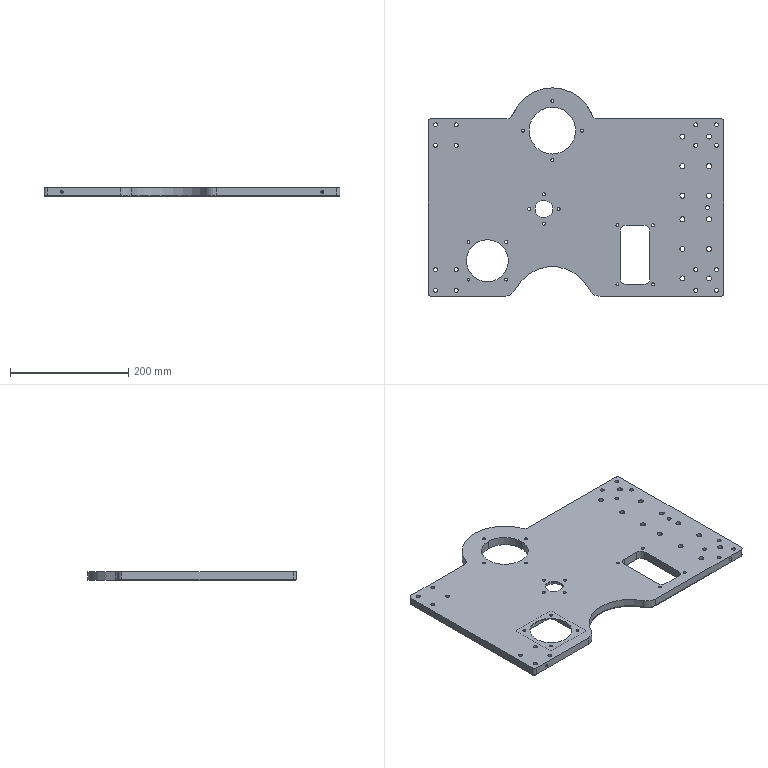NC program | Mastercam | posted with a generic post
Lines 1 to 790 of 11903:
%
O0000()
(MATERIAL - ALUMINUM MM - 2024)
( T20 | 20 FEM | H20 | XY STOCK TO LEAVE - .1 | Z STOCK TO LEAVE - .03 )
( T16 | 16 FEM | H16 | XY STOCK TO LEAVE - 0. | Z STOCK TO LEAVE - .03 )
( T8 | 8 FEM | H8 | XY STOCK TO LEAVE - .1 | Z STOCK TO LEAVE - .2 )
( T4 | 4 FEM | H4 | XY STOCK TO LEAVE - .05 | Z STOCK TO LEAVE - .2 )
( T7 | 4 CHM | H7 )
( T18 | 8.5 DR | H18 )
( T14 | 6.8 DR | H14 )
( T1 | 5 DR | H1 )
( T9 | 6.6 DR | H9 )
( T6 | 6 FEM | H6 | XY STOCK TO LEAVE - .07 | Z STOCK TO LEAVE - .05 )
( T11 | 8 BNOS | H11 )
( T3 | 10.5 DR | H3 )
N100 G21
N110 G0 G17 G40 G49 G80 G90
( YDICL )
N120 T20 M6
N130 G0 G90 G54 X260.1 Y191.25 A0. S5000 M3
N140 G43 H20 Z50. M8
N150 Z1.1
N160 G1 Z-1.784 F600.
N170 Y171.25 F4000.
N180 Y-171.75
N190 Y-191.75
N200 Z-3.667 F600.
N210 Y-171.75 F4000.
N220 Y171.25
N230 Y191.25
N240 Z-5.551 F600.
N250 Y171.25 F4000.
N260 Y-171.75
N270 Y-191.75
N280 Z-7.435 F600.
N290 Y-171.75 F4000.
N300 Y171.25
N310 Y191.25
N320 Z-9.319 F600.
N330 Y171.25 F4000.
N340 Y-171.75
N350 Y-191.75
N360 Z-11.203 F600.
N370 Y-171.75 F4000.
N380 Y171.25
N390 Y191.25
N400 Z-13.086 F600.
N410 Y171.25 F4000.
N420 Y-171.75
N430 Y-191.75
N440 Z-14.97 F600.
N450 Y-171.75 F4000.
N460 Y171.25
N470 Y191.25
N480 G0 Z50.
N490 X-260.1 Y-191.75
N500 Z1.1
N510 G1 Z-1.784 F600.
N520 Y-171.75 F4000.
N530 Y171.25
N540 Y191.25
N550 Z-3.667 F600.
N560 Y171.25 F4000.
N570 Y-171.75
N580 Y-191.75
N590 Z-5.551 F600.
N600 Y-171.75 F4000.
N610 Y171.25
N620 Y191.25
N630 Z-7.435 F600.
N640 Y171.25 F4000.
N650 Y-171.75
N660 Y-191.75
N670 Z-9.319 F600.
N680 Y-171.75 F4000.
N690 Y171.25
N700 Y191.25
N710 Z-11.203 F600.
N720 Y171.25 F4000.
N730 Y-171.75
N740 Y-191.75
N750 Z-13.086 F600.
N760 Y-171.75 F4000.
N770 Y171.25
N780 Y191.25
N790 Z-14.97 F600.
N800 Y171.25 F4000.
N810 Y-171.75
N820 Y-191.75
N830 G0 Z50.
N840 X-40. Y-93.85
N850 Z1.1
N860 G1 Z.1 F600.
N870 G3 X-49.9 Y-103.75 Z-.15 I0. J-9.9 F4000.
N880 X-40. Y-113.65 Z-.4 I9.9 J0.
N890 X-30.1 Y-103.75 Z-.65 I0. J9.9
N900 X-40. Y-93.85 Z-.9 I-9.9 J0.
N910 X-49.9 Y-103.75 Z-1.15 I0. J-9.9
N920 X-40. Y-113.65 Z-1.4 I9.9 J0.
N930 X-30.1 Y-103.75 Z-1.65 I0. J9.9
N940 X-40. Y-93.85 Z-1.9 I-9.9 J0.
N950 X-49.9 Y-103.75 Z-2.15 I0. J-9.9
N960 X-40. Y-113.65 Z-2.4 I9.9 J0.
N970 X-30.1 Y-103.75 Z-2.65 I0. J9.9
N980 X-40. Y-93.85 Z-2.9 I-9.9 J0.
N990 X-49.9 Y-103.75 Z-3.15 I0. J-9.9
N1000 X-40. Y-113.65 Z-3.4 I9.9 J0.
N1010 X-30.1 Y-103.75 Z-3.65 I0. J9.9
N1020 X-40. Y-93.85 Z-3.9 I-9.9 J0.
N1030 X-49.9 Y-103.75 Z-4.15 I0. J-9.9
N1040 X-40. Y-113.65 Z-4.4 I9.9 J0.
N1050 X-30.1 Y-103.75 Z-4.65 I0. J9.9
N1060 X-40. Y-93.85 Z-4.9 I-9.9 J0.
N1070 X-49.9 Y-103.75 Z-5.15 I0. J-9.9
N1080 X-40. Y-113.65 Z-5.4 I9.9 J0.
N1090 X-30.1 Y-103.75 Z-5.65 I0. J9.9
N1100 X-40. Y-93.85 Z-5.9 I-9.9 J0.
N1110 X-49.9 Y-103.75 Z-6.15 I0. J-9.9
N1120 X-40. Y-113.65 Z-6.4 I9.9 J0.
N1130 X-30.1 Y-103.75 Z-6.65 I0. J9.9
N1140 X-40. Y-93.85 Z-6.9 I-9.9 J0.
N1150 X-49.9 Y-103.75 Z-7.15 I0. J-9.9
N1160 X-40. Y-113.65 Z-7.4 I9.9 J0.
N1170 X-30.1 Y-103.75 Z-7.65 I0. J9.9
N1180 X-40. Y-93.85 Z-7.9 I-9.9 J0.
N1190 X-49.9 Y-103.75 Z-8.15 I0. J-9.9
N1200 X-40. Y-113.65 Z-8.4 I9.9 J0.
N1210 X-30.1 Y-103.75 Z-8.65 I0. J9.9
N1220 X-40. Y-93.85 Z-8.9 I-9.9 J0.
N1230 X-49.9 Y-103.75 Z-9.15 I0. J-9.9
N1240 X-40. Y-113.65 Z-9.4 I9.9 J0.
N1250 X-30.1 Y-103.75 Z-9.65 I0. J9.9
N1260 X-40. Y-93.85 Z-9.9 I-9.9 J0.
N1270 X-49.9 Y-103.75 Z-10.15 I0. J-9.9
N1280 X-40. Y-113.65 Z-10.4 I9.9 J0.
N1290 X-30.1 Y-103.75 Z-10.65 I0. J9.9
N1300 X-40. Y-93.85 Z-10.9 I-9.9 J0.
N1310 X-49.9 Y-103.75 Z-11.15 I0. J-9.9
N1320 X-40. Y-113.65 Z-11.4 I9.9 J0.
N1330 X-30.1 Y-103.75 Z-11.65 I0. J9.9
N1340 X-40. Y-93.85 Z-11.9 I-9.9 J0.
N1350 X-49.9 Y-103.75 Z-12.15 I0. J-9.9
N1360 X-40. Y-113.65 Z-12.4 I9.9 J0.
N1370 X-30.1 Y-103.75 Z-12.65 I0. J9.9
N1380 X-40. Y-93.85 Z-12.9 I-9.9 J0.
N1390 X-49.9 Y-103.75 Z-13.15 I0. J-9.9
N1400 X-40. Y-113.65 Z-13.4 I9.9 J0.
N1410 X-30.1 Y-103.75 Z-13.65 I0. J9.9
N1420 X-40. Y-93.85 Z-13.9 I-9.9 J0.
N1430 X-49.9 Y-103.75 Z-14.15 I0. J-9.9
N1440 X-40. Y-113.65 Z-14.4 I9.9 J0.
N1450 X-30.1 Y-103.75 Z-14.65 I0. J9.9
N1460 X-40. Y-93.85 Z-14.9 I-9.9 J0.
N1470 X-44.215 Y-94.792 Z-14.97 I0. J-9.9
N1480 X-49.9 Y-103.75 I4.215 J-8.958
N1490 X-40. Y-113.65 I9.9 J0.
N1500 X-30.1 Y-103.75 I0. J9.9
N1510 X-40. Y-93.85 I-9.9 J0.
N1520 X-44.662 Y-95.016 I0. J-9.9
N1530 G0 Z50.
N1540 X-40. Y-74.35
N1550 Z1.1
N1560 G1 Z.1 F600.
N1570 G3 X-69.4 Y-103.75 Z-.15 I0. J-29.4 F4000.
N1580 X-40. Y-133.15 Z-.4 I29.4 J0.
N1590 X-10.6 Y-103.75 Z-.65 I0. J29.4
N1600 X-40. Y-74.35 Z-.9 I-29.4 J0.
N1610 X-69.4 Y-103.75 Z-1.15 I0. J-29.4
N1620 X-40. Y-133.15 Z-1.4 I29.4 J0.
N1630 X-10.6 Y-103.75 Z-1.65 I0. J29.4
N1640 X-40. Y-74.35 Z-1.9 I-29.4 J0.
N1650 X-69.4 Y-103.75 Z-2.15 I0. J-29.4
N1660 X-40. Y-133.15 Z-2.4 I29.4 J0.
N1670 X-10.6 Y-103.75 Z-2.65 I0. J29.4
N1680 X-40. Y-74.35 Z-2.9 I-29.4 J0.
N1690 X-69.4 Y-103.75 Z-3.15 I0. J-29.4
N1700 X-40. Y-133.15 Z-3.4 I29.4 J0.
N1710 X-10.6 Y-103.75 Z-3.65 I0. J29.4
N1720 X-40. Y-74.35 Z-3.9 I-29.4 J0.
N1730 X-69.4 Y-103.75 Z-4.15 I0. J-29.4
N1740 X-40. Y-133.15 Z-4.4 I29.4 J0.
N1750 X-10.6 Y-103.75 Z-4.65 I0. J29.4
N1760 X-40. Y-74.35 Z-4.9 I-29.4 J0.
N1770 X-69.4 Y-103.75 Z-5.15 I0. J-29.4
N1780 X-40. Y-133.15 Z-5.4 I29.4 J0.
N1790 X-10.6 Y-103.75 Z-5.65 I0. J29.4
N1800 X-40. Y-74.35 Z-5.9 I-29.4 J0.
N1810 X-69.4 Y-103.75 Z-6.15 I0. J-29.4
N1820 X-40. Y-133.15 Z-6.4 I29.4 J0.
N1830 X-10.6 Y-103.75 Z-6.65 I0. J29.4
N1840 X-40. Y-74.35 Z-6.9 I-29.4 J0.
N1850 X-69.4 Y-103.75 Z-7.15 I0. J-29.4
N1860 X-40. Y-133.15 Z-7.4 I29.4 J0.
N1870 X-10.6 Y-103.75 Z-7.65 I0. J29.4
N1880 X-40. Y-74.35 Z-7.9 I-29.4 J0.
N1890 X-69.4 Y-103.75 Z-8.15 I0. J-29.4
N1900 X-40. Y-133.15 Z-8.4 I29.4 J0.
N1910 X-10.6 Y-103.75 Z-8.65 I0. J29.4
N1920 X-40. Y-74.35 Z-8.9 I-29.4 J0.
N1930 X-69.4 Y-103.75 Z-9.15 I0. J-29.4
N1940 X-40. Y-133.15 Z-9.4 I29.4 J0.
N1950 X-10.6 Y-103.75 Z-9.65 I0. J29.4
N1960 X-40. Y-74.35 Z-9.9 I-29.4 J0.
N1970 X-69.4 Y-103.75 Z-10.15 I0. J-29.4
N1980 X-40. Y-133.15 Z-10.4 I29.4 J0.
N1990 X-10.6 Y-103.75 Z-10.65 I0. J29.4
N2000 X-40. Y-74.35 Z-10.9 I-29.4 J0.
N2010 X-69.4 Y-103.75 Z-11.15 I0. J-29.4
N2020 X-40. Y-133.15 Z-11.4 I29.4 J0.
N2030 X-10.6 Y-103.75 Z-11.65 I0. J29.4
N2040 X-40. Y-74.35 Z-11.9 I-29.4 J0.
N2050 X-69.4 Y-103.75 Z-12.15 I0. J-29.4
N2060 X-40. Y-133.15 Z-12.4 I29.4 J0.
N2070 X-10.6 Y-103.75 Z-12.65 I0. J29.4
N2080 X-40. Y-74.35 Z-12.9 I-29.4 J0.
N2090 X-69.4 Y-103.75 Z-13.15 I0. J-29.4
N2100 X-40. Y-133.15 Z-13.4 I29.4 J0.
N2110 X-10.6 Y-103.75 Z-13.65 I0. J29.4
N2120 X-40. Y-74.35 Z-13.9 I-29.4 J0.
N2130 X-69.4 Y-103.75 Z-14.15 I0. J-29.4
N2140 X-40. Y-133.15 Z-14.4 I29.4 J0.
N2150 X-10.6 Y-103.75 Z-14.65 I0. J29.4
N2160 X-40. Y-74.35 Z-14.9 I-29.4 J0.
N2170 X-52.518 Y-77.148 Z-14.97 I0. J-29.4
N2180 X-69.4 Y-103.75 I12.518 J-26.602
N2190 X-40. Y-133.15 I29.4 J0.
N2200 X-10.6 Y-103.75 I0. J29.4
N2210 X-40. Y-74.35 I-29.4 J0.
N2220 X-52.968 Y-77.365 I0. J-29.4
N2230 G0 Z50.
N2240 X106.9 Y138.15
N2250 Z1.1
N2260 G1 Z.1 F600.
N2270 X93.1 Z.011 F4000.
N2280 Y74.35 Z-.4
N2290 X106.9 Z-.489
N2300 Y138.15 Z-.9
N2310 X93.1 Z-.989
N2320 Y74.35 Z-1.4
N2330 X106.9 Z-1.489
N2340 Y138.15 Z-1.9
N2350 X93.1 Z-1.989
N2360 Y74.35 Z-2.4
N2370 X106.9 Z-2.489
N2380 Y138.15 Z-2.9
N2390 X93.1 Z-2.989
N2400 Y74.35 Z-3.4
N2410 X106.9 Z-3.489
N2420 Y138.15 Z-3.9
N2430 X93.1 Z-3.989
N2440 Y74.35 Z-4.4
N2450 X106.9 Z-4.489
N2460 Y138.15 Z-4.9
N2470 X93.1 Z-4.989
N2480 Y74.35 Z-5.4
N2490 X106.9 Z-5.489
N2500 Y138.15 Z-5.9
N2510 X93.1 Z-5.989
N2520 Y74.35 Z-6.4
N2530 X106.9 Z-6.489
N2540 Y138.15 Z-6.9
N2550 X93.1 Z-6.989
N2560 Y74.35 Z-7.4
N2570 X106.9 Z-7.489
N2580 Y138.15 Z-7.9
N2590 X93.1 Z-7.989
N2600 Y74.35 Z-8.4
N2610 X106.9 Z-8.489
N2620 Y138.15 Z-8.9
N2630 X93.1 Z-8.989
N2640 Y74.35 Z-9.4
N2650 X106.9 Z-9.489
N2660 Y138.15 Z-9.9
N2670 X93.1 Z-9.989
N2680 Y74.35 Z-10.4
N2690 X106.9 Z-10.489
N2700 Y138.15 Z-10.9
N2710 X93.1 Z-10.989
N2720 Y74.35 Z-11.4
N2730 X106.9 Z-11.489
N2740 Y138.15 Z-11.9
N2750 X93.1 Z-11.989
N2760 Y74.35 Z-12.4
N2770 X106.9 Z-12.489
N2780 Y138.15 Z-12.9
N2790 X93.1 Z-12.989
N2800 Y74.35 Z-13.4
N2810 X106.9 Z-13.489
N2820 Y138.15 Z-13.9
N2830 X93.1 Z-13.989
N2840 Y74.35 Z-14.4
N2850 X106.9 Z-14.489
N2860 Y138.15 Z-14.9
N2870 X96.036 Z-14.97
N2880 X93.1
N2890 Y74.35
N2900 X106.9
N2910 Y138.15
N2920 X95.536
N2930 G0 Z50.
N2940 X114.9 Y146.15
N2950 Z1.1
N2960 G1 Z.1 F600.
N2970 X85.1 Z-.036 F4000.
N2980 Y66.35 Z-.4
N2990 X114.9 Z-.536
N3000 Y146.15 Z-.9
N3010 X85.1 Z-1.036
N3020 Y66.35 Z-1.4
N3030 X114.9 Z-1.536
N3040 Y146.15 Z-1.9
N3050 X85.1 Z-2.036
N3060 Y66.35 Z-2.4
N3070 X114.9 Z-2.536
N3080 Y146.15 Z-2.9
N3090 X85.1 Z-3.036
N3100 Y66.35 Z-3.4
N3110 X114.9 Z-3.536
N3120 Y146.15 Z-3.9
N3130 X85.1 Z-4.036
N3140 Y66.35 Z-4.4
N3150 X114.9 Z-4.536
N3160 Y146.15 Z-4.9
N3170 X85.1 Z-5.036
N3180 Y66.35 Z-5.4
N3190 X114.9 Z-5.536
N3200 Y146.15 Z-5.9
N3210 X85.1 Z-6.036
N3220 Y66.35 Z-6.4
N3230 X114.9 Z-6.536
N3240 Y146.15 Z-6.9
N3250 X85.1 Z-7.036
N3260 Y66.35 Z-7.4
N3270 X114.9 Z-7.536
N3280 Y146.15 Z-7.9
N3290 X85.1 Z-8.036
N3300 Y66.35 Z-8.4
N3310 X114.9 Z-8.536
N3320 Y146.15 Z-8.9
N3330 X85.1 Z-9.036
N3340 Y66.35 Z-9.4
N3350 X114.9 Z-9.536
N3360 Y146.15 Z-9.9
N3370 X85.1 Z-10.036
N3380 Y66.35 Z-10.4
N3390 X114.9 Z-10.536
N3400 Y146.15 Z-10.9
N3410 X85.1 Z-11.036
N3420 Y66.35 Z-11.4
N3430 X114.9 Z-11.536
N3440 Y146.15 Z-11.9
N3450 X85.1 Z-12.036
N3460 Y66.35 Z-12.4
N3470 X114.9 Z-12.536
N3480 Y146.15 Z-12.9
N3490 X85.1 Z-13.036
N3500 Y66.35 Z-13.4
N3510 X114.9 Z-13.536
N3520 Y146.15 Z-13.9
N3530 X85.1 Z-14.036
N3540 Y66.35 Z-14.4
N3550 X114.9 Z-14.536
N3560 Y146.15 Z-14.9
N3570 X99.556 Z-14.97
N3580 X85.1
N3590 Y66.35
N3600 X114.9
N3610 Y146.15
N3620 X99.056
N3630 G0 Z50.
N3640 X-54.364 Y33.668
N3650 Z1.1
N3660 G1 Z.1 F600.
N3670 G3 X-59.264 Y28.768 Z-.15 I0. J-4.9 F3000.
N3680 X-54.364 Y23.868 Z-.4 I4.9 J0.
N3690 X-49.464 Y28.768 Z-.65 I0. J4.9
N3700 X-54.364 Y33.668 Z-.9 I-4.9 J0.
N3710 X-59.264 Y28.768 Z-1.15 I0. J-4.9
N3720 X-54.364 Y23.868 Z-1.4 I4.9 J0.
N3730 X-49.464 Y28.768 Z-1.65 I0. J4.9
N3740 X-54.364 Y33.668 Z-1.9 I-4.9 J0.
N3750 X-59.264 Y28.768 Z-2.15 I0. J-4.9
N3760 X-54.364 Y23.868 Z-2.4 I4.9 J0.
N3770 X-49.464 Y28.768 Z-2.65 I0. J4.9
N3780 X-54.364 Y33.668 Z-2.9 I-4.9 J0.
N3790 X-59.264 Y28.768 Z-3.15 I0. J-4.9
N3800 X-54.364 Y23.868 Z-3.4 I4.9 J0.
N3810 X-49.464 Y28.768 Z-3.65 I0. J4.9
N3820 X-54.364 Y33.668 Z-3.9 I-4.9 J0.
N3830 X-59.264 Y28.768 Z-4.15 I0. J-4.9
N3840 X-54.364 Y23.868 Z-4.4 I4.9 J0.
N3850 X-49.464 Y28.768 Z-4.65 I0. J4.9
N3860 X-54.364 Y33.668 Z-4.9 I-4.9 J0.
N3870 X-59.264 Y28.768 Z-5.15 I0. J-4.9
N3880 X-54.364 Y23.868 Z-5.4 I4.9 J0.
N3890 X-49.464 Y28.768 Z-5.65 I0. J4.9
N3900 X-54.364 Y33.668 Z-5.9 I-4.9 J0.
N3910 X-59.264 Y28.768 Z-6.15 I0. J-4.9
N3920 X-54.364 Y23.868 Z-6.4 I4.9 J0.
N3930 X-49.464 Y28.768 Z-6.65 I0. J4.9
N3940 X-54.364 Y33.668 Z-6.9 I-4.9 J0.
N3950 X-59.264 Y28.768 Z-7.15 I0. J-4.9
N3960 X-54.364 Y23.868 Z-7.4 I4.9 J0.
N3970 X-49.464 Y28.768 Z-7.65 I0. J4.9
N3980 X-54.364 Y33.668 Z-7.9 I-4.9 J0.
N3990 X-59.264 Y28.768 Z-8.15 I0. J-4.9
N4000 X-54.364 Y23.868 Z-8.4 I4.9 J0.
N4010 X-49.464 Y28.768 Z-8.65 I0. J4.9
N4020 X-54.364 Y33.668 Z-8.9 I-4.9 J0.
N4030 X-59.264 Y28.768 Z-9.15 I0. J-4.9
N4040 X-54.364 Y23.868 Z-9.4 I4.9 J0.
N4050 X-49.464 Y28.768 Z-9.65 I0. J4.9
N4060 X-54.364 Y33.668 Z-9.9 I-4.9 J0.
N4070 X-59.264 Y28.768 Z-10.15 I0. J-4.9
N4080 X-54.364 Y23.868 Z-10.4 I4.9 J0.
N4090 X-49.464 Y28.768 Z-10.65 I0. J4.9
N4100 X-54.364 Y33.668 Z-10.9 I-4.9 J0.
N4110 X-59.264 Y28.768 Z-11.15 I0. J-4.9
N4120 X-54.364 Y23.868 Z-11.4 I4.9 J0.
N4130 X-49.464 Y28.768 Z-11.65 I0. J4.9
N4140 X-54.364 Y33.668 Z-11.9 I-4.9 J0.
N4150 X-59.264 Y28.768 Z-12.15 I0. J-4.9
N4160 X-54.364 Y23.868 Z-12.4 I4.9 J0.
N4170 X-49.464 Y28.768 Z-12.65 I0. J4.9
N4180 X-54.364 Y33.668 Z-12.9 I-4.9 J0.
N4190 X-59.264 Y28.768 Z-13.15 I0. J-4.9
N4200 X-54.364 Y23.868 Z-13.4 I4.9 J0.
N4210 X-49.464 Y28.768 Z-13.65 I0. J4.9
N4220 X-54.364 Y33.668 Z-13.9 I-4.9 J0.
N4230 X-59.264 Y28.768 Z-14.15 I0. J-4.9
N4240 X-54.364 Y23.868 Z-14.4 I4.9 J0.
N4250 X-49.464 Y28.768 Z-14.65 I0. J4.9
N4260 X-54.364 Y33.668 Z-14.9 I-4.9 J0.
N4270 X-56.45 Y33.201 Z-14.97 I0. J-4.9
N4280 X-59.263 Y28.768 I2.086 J-4.433
N4290 X-54.364 Y23.869 I4.899 J0.
N4300 X-49.465 Y28.768 I0. J4.899
N4310 X-54.364 Y33.668 I-4.899 J0.
N4320 X-56.891 Y32.966 I0. J-4.9
N4330 G0 Z50.
N4340 X-54.364 Y37.168
N4350 Z1.1
N4360 G1 Z.1 F600.
N4370 G3 X-62.764 Y28.768 Z-.15 I0. J-8.4 F3000.
N4380 X-54.364 Y20.368 Z-.4 I8.4 J0.
N4390 X-45.964 Y28.768 Z-.65 I0. J8.4
N4400 X-54.364 Y37.168 Z-.9 I-8.4 J0.
N4410 X-62.764 Y28.768 Z-1.15 I0. J-8.4
N4420 X-54.364 Y20.368 Z-1.4 I8.4 J0.
N4430 X-45.964 Y28.768 Z-1.65 I0. J8.4
N4440 X-54.364 Y37.168 Z-1.9 I-8.4 J0.
N4450 X-62.764 Y28.768 Z-2.15 I0. J-8.4
N4460 X-54.364 Y20.368 Z-2.4 I8.4 J0.
N4470 X-45.964 Y28.768 Z-2.65 I0. J8.4
N4480 X-54.364 Y37.168 Z-2.9 I-8.4 J0.
N4490 X-62.764 Y28.768 Z-3.15 I0. J-8.4
N4500 X-54.364 Y20.368 Z-3.4 I8.4 J0.
N4510 X-45.964 Y28.768 Z-3.65 I0. J8.4
N4520 X-54.364 Y37.168 Z-3.9 I-8.4 J0.
N4530 X-62.764 Y28.768 Z-4.15 I0. J-8.4
N4540 X-54.364 Y20.368 Z-4.4 I8.4 J0.
N4550 X-45.964 Y28.768 Z-4.65 I0. J8.4
N4560 X-54.364 Y37.168 Z-4.9 I-8.4 J0.
N4570 X-62.764 Y28.768 Z-5.15 I0. J-8.4
N4580 X-54.364 Y20.368 Z-5.4 I8.4 J0.
N4590 X-45.964 Y28.768 Z-5.65 I0. J8.4
N4600 X-54.364 Y37.168 Z-5.9 I-8.4 J0.
N4610 X-62.764 Y28.768 Z-6.15 I0. J-8.4
N4620 X-54.364 Y20.368 Z-6.4 I8.4 J0.
N4630 X-45.964 Y28.768 Z-6.65 I0. J8.4
N4640 X-54.364 Y37.168 Z-6.9 I-8.4 J0.
N4650 X-62.764 Y28.768 Z-7.15 I0. J-8.4
N4660 X-54.364 Y20.368 Z-7.4 I8.4 J0.
N4670 X-45.964 Y28.768 Z-7.65 I0. J8.4
N4680 X-54.364 Y37.168 Z-7.9 I-8.4 J0.
N4690 X-62.764 Y28.768 Z-8.15 I0. J-8.4
N4700 X-54.364 Y20.368 Z-8.4 I8.4 J0.
N4710 X-45.964 Y28.768 Z-8.65 I0. J8.4
N4720 X-54.364 Y37.168 Z-8.9 I-8.4 J0.
N4730 X-62.764 Y28.768 Z-9.15 I0. J-8.4
N4740 X-54.364 Y20.368 Z-9.4 I8.4 J0.
N4750 X-45.964 Y28.768 Z-9.65 I0. J8.4
N4760 X-54.364 Y37.168 Z-9.9 I-8.4 J0.
N4770 X-62.764 Y28.768 Z-10.15 I0. J-8.4
N4780 X-54.364 Y20.368 Z-10.4 I8.4 J0.
N4790 X-45.964 Y28.768 Z-10.65 I0. J8.4
N4800 X-54.364 Y37.168 Z-10.9 I-8.4 J0.
N4810 X-62.764 Y28.768 Z-11.15 I0. J-8.4
N4820 X-54.364 Y20.368 Z-11.4 I8.4 J0.
N4830 X-45.964 Y28.768 Z-11.65 I0. J8.4
N4840 X-54.364 Y37.168 Z-11.9 I-8.4 J0.
N4850 X-62.764 Y28.768 Z-12.15 I0. J-8.4
N4860 X-54.364 Y20.368 Z-12.4 I8.4 J0.
N4870 X-45.964 Y28.768 Z-12.65 I0. J8.4
N4880 X-54.364 Y37.168 Z-12.9 I-8.4 J0.
N4890 X-62.764 Y28.768 I0. J-8.4
N4900 X-54.364 Y20.368 I8.4 J0.
N4910 X-45.964 Y28.768 I0. J8.4
N4920 X-54.364 Y37.168 I-8.4 J0.
N4930 X-54.863 Y37.153 I0. J-8.4
N4940 G0 Z50.
N4950 X-54.364 Y52.668
N4960 Z1.3
N4970 G1 Z.3 F600.
N4980 G3 X-78.264 Y28.768 Z.05 I0. J-23.9 F4000.
N4990 X-54.364 Y4.868 Z-.2 I23.9 J0.
N5000 X-30.464 Y28.768 Z-.45 I0. J23.9
N5010 X-54.364 Y52.668 Z-.7 I-23.9 J0.
N5020 X-78.264 Y28.768 Z-.95 I0. J-23.9
N5030 X-54.364 Y4.868 Z-1.2 I23.9 J0.
N5040 X-30.464 Y28.768 Z-1.45 I0. J23.9
N5050 X-54.364 Y52.668 Z-1.7 I-23.9 J0.
N5060 X-78.264 Y28.768 Z-1.95 I0. J-23.9
N5070 X-54.364 Y4.868 Z-2.2 I23.9 J0.
N5080 X-30.464 Y28.768 Z-2.45 I0. J23.9
N5090 X-54.364 Y52.668 Z-2.7 I-23.9 J0.
N5100 X-78.264 Y28.768 Z-2.95 I0. J-23.9
N5110 X-54.364 Y4.868 Z-3.2 I23.9 J0.
N5120 X-30.464 Y28.768 Z-3.45 I0. J23.9
N5130 X-54.364 Y52.668 Z-3.7 I-23.9 J0.
N5140 X-78.264 Y28.768 Z-3.95 I0. J-23.9
N5150 X-54.364 Y4.868 Z-4.2 I23.9 J0.
N5160 X-30.464 Y28.768 Z-4.45 I0. J23.9
N5170 X-54.364 Y52.668 Z-4.7 I-23.9 J0.
N5180 X-78.264 Y28.768 Z-4.95 I0. J-23.9
N5190 X-54.364 Y4.868 Z-5.2 I23.9 J0.
N5200 X-30.464 Y28.768 Z-5.45 I0. J23.9
N5210 X-54.364 Y52.668 Z-5.7 I-23.9 J0.
N5220 X-78.264 Y28.768 Z-5.95 I0. J-23.9
N5230 X-54.364 Y4.868 Z-6.2 I23.9 J0.
N5240 X-30.464 Y28.768 Z-6.45 I0. J23.9
N5250 X-54.364 Y52.668 Z-6.7 I-23.9 J0.
N5260 X-77.094 Y36.153 Z-6.9 I0. J-23.9
N5270 X-78.264 Y28.768 I22.73 J-7.385
N5280 X-54.364 Y4.868 I23.9 J0.
N5290 X-30.464 Y28.768 I0. J23.9
N5300 X-54.364 Y52.668 I-23.9 J0.
N5310 X-77.243 Y35.676 I0. J-23.9
N5320 G0 Z50.
N5330 X-150. Y124.65
N5340 Z1.1
N5350 G1 Z.1 F600.
N5360 G3 X-158.4 Y116.25 Z-.15 I0. J-8.4 F4000.
N5370 X-150. Y107.85 Z-.4 I8.4 J0.
N5380 X-141.6 Y116.25 Z-.65 I0. J8.4
N5390 X-150. Y124.65 Z-.9 I-8.4 J0.
N5400 X-158.4 Y116.25 Z-1.15 I0. J-8.4
N5410 X-150. Y107.85 Z-1.4 I8.4 J0.
N5420 X-141.6 Y116.25 Z-1.65 I0. J8.4
N5430 X-150. Y124.65 Z-1.9 I-8.4 J0.
N5440 X-158.4 Y116.25 Z-2.15 I0. J-8.4
N5450 X-150. Y107.85 Z-2.4 I8.4 J0.
N5460 X-141.6 Y116.25 Z-2.65 I0. J8.4
N5470 X-150. Y124.65 Z-2.9 I-8.4 J0.
N5480 X-158.4 Y116.25 Z-3.15 I0. J-8.4
N5490 X-150. Y107.85 Z-3.4 I8.4 J0.
N5500 X-141.6 Y116.25 Z-3.65 I0. J8.4
N5510 X-150. Y124.65 Z-3.9 I-8.4 J0.
N5520 X-158.4 Y116.25 Z-4.15 I0. J-8.4
N5530 X-150. Y107.85 Z-4.4 I8.4 J0.
N5540 X-141.6 Y116.25 Z-4.65 I0. J8.4
N5550 X-150. Y124.65 Z-4.9 I-8.4 J0.
N5560 X-158.4 Y116.25 Z-5.15 I0. J-8.4
N5570 X-150. Y107.85 Z-5.4 I8.4 J0.
N5580 X-141.6 Y116.25 Z-5.65 I0. J8.4
N5590 X-150. Y124.65 Z-5.9 I-8.4 J0.
N5600 X-158.4 Y116.25 Z-6.15 I0. J-8.4
N5610 X-150. Y107.85 Z-6.4 I8.4 J0.
N5620 X-141.6 Y116.25 Z-6.65 I0. J8.4
N5630 X-150. Y124.65 Z-6.9 I-8.4 J0.
N5640 X-158.4 Y116.25 Z-7.15 I0. J-8.4
N5650 X-150. Y107.85 Z-7.4 I8.4 J0.
N5660 X-141.6 Y116.25 Z-7.65 I0. J8.4
N5670 X-150. Y124.65 Z-7.9 I-8.4 J0.
N5680 X-158.4 Y116.25 Z-8.15 I0. J-8.4
N5690 X-150. Y107.85 Z-8.4 I8.4 J0.
N5700 X-141.6 Y116.25 Z-8.65 I0. J8.4
N5710 X-150. Y124.65 Z-8.9 I-8.4 J0.
N5720 X-158.4 Y116.25 Z-9.15 I0. J-8.4
N5730 X-150. Y107.85 Z-9.4 I8.4 J0.
N5740 X-141.6 Y116.25 Z-9.65 I0. J8.4
N5750 X-150. Y124.65 Z-9.9 I-8.4 J0.
N5760 X-158.4 Y116.25 Z-10.15 I0. J-8.4
N5770 X-150. Y107.85 Z-10.4 I8.4 J0.
N5780 X-141.6 Y116.25 Z-10.65 I0. J8.4
N5790 X-150. Y124.65 Z-10.9 I-8.4 J0.
N5800 X-158.4 Y116.25 Z-11.15 I0. J-8.4
N5810 X-150. Y107.85 Z-11.4 I8.4 J0.
N5820 X-141.6 Y116.25 Z-11.65 I0. J8.4
N5830 X-150. Y124.65 Z-11.9 I-8.4 J0.
N5840 X-158.4 Y116.25 Z-12.15 I0. J-8.4
N5850 X-150. Y107.85 Z-12.4 I8.4 J0.
N5860 X-141.6 Y116.25 Z-12.65 I0. J8.4
N5870 X-150. Y124.65 Z-12.9 I-8.4 J0.
N5880 X-158.4 Y116.25 Z-13.15 I0. J-8.4
N5890 X-150. Y107.85 Z-13.4 I8.4 J0.
N5900 X-141.6 Y116.25 Z-13.65 I0. J8.4
N5910 X-150. Y124.65 Z-13.9 I-8.4 J0.
N5920 X-158.4 Y116.25 Z-14.15 I0. J-8.4
N5930 X-150. Y107.85 Z-14.4 I8.4 J0.
N5940 X-141.6 Y116.25 Z-14.65 I0. J8.4
N5950 X-150. Y124.65 Z-14.9 I-8.4 J0.
N5960 X-153.577 Y123.851 Z-14.97 I0. J-8.4
N5970 X-158.401 Y116.25 I3.577 J-7.601
N5980 X-150. Y107.849 I8.401 J0.
N5990 X-141.599 Y116.25 I0. J8.401
N6000 X-150. Y124.65 I-8.401 J0.
N6010 X-154.022 Y123.624 I0. J-8.4
N6020 G0 Z50.
N6030 X-150. Y141.65
N6040 Z1.1
N6050 G1 Z.1 F600.
N6060 G3 X-175.4 Y116.25 Z-.15 I0. J-25.4 F4000.
N6070 X-150. Y90.85 Z-.4 I25.4 J0.
N6080 X-124.6 Y116.25 Z-.65 I0. J25.4
N6090 X-150. Y141.65 Z-.9 I-25.4 J0.
N6100 X-175.4 Y116.25 Z-1.15 I0. J-25.4
N6110 X-150. Y90.85 Z-1.4 I25.4 J0.
N6120 X-124.6 Y116.25 Z-1.65 I0. J25.4
N6130 X-150. Y141.65 Z-1.9 I-25.4 J0.
N6140 X-175.4 Y116.25 Z-2.15 I0. J-25.4
N6150 X-150. Y90.85 Z-2.4 I25.4 J0.
N6160 X-124.6 Y116.25 Z-2.65 I0. J25.4
N6170 X-150. Y141.65 Z-2.9 I-25.4 J0.
N6180 X-175.4 Y116.25 Z-3.15 I0. J-25.4
N6190 X-150. Y90.85 Z-3.4 I25.4 J0.
N6200 X-124.6 Y116.25 Z-3.65 I0. J25.4
N6210 X-150. Y141.65 Z-3.9 I-25.4 J0.
N6220 X-175.4 Y116.25 Z-4.15 I0. J-25.4
N6230 X-150. Y90.85 Z-4.4 I25.4 J0.
N6240 X-124.6 Y116.25 Z-4.65 I0. J25.4
N6250 X-150. Y141.65 Z-4.9 I-25.4 J0.
N6260 X-175.4 Y116.25 Z-5.15 I0. J-25.4
N6270 X-150. Y90.85 Z-5.4 I25.4 J0.
N6280 X-124.6 Y116.25 Z-5.65 I0. J25.4
N6290 X-150. Y141.65 Z-5.9 I-25.4 J0.
N6300 X-175.4 Y116.25 Z-6.15 I0. J-25.4
N6310 X-150. Y90.85 Z-6.4 I25.4 J0.
N6320 X-124.6 Y116.25 Z-6.65 I0. J25.4
N6330 X-150. Y141.65 Z-6.9 I-25.4 J0.
N6340 X-175.4 Y116.25 Z-7.15 I0. J-25.4
N6350 X-150. Y90.85 Z-7.4 I25.4 J0.
N6360 X-124.6 Y116.25 Z-7.65 I0. J25.4
N6370 X-150. Y141.65 Z-7.9 I-25.4 J0.
N6380 X-175.4 Y116.25 Z-8.15 I0. J-25.4
N6390 X-150. Y90.85 Z-8.4 I25.4 J0.
N6400 X-124.6 Y116.25 Z-8.65 I0. J25.4
N6410 X-150. Y141.65 Z-8.9 I-25.4 J0.
N6420 X-175.4 Y116.25 Z-9.15 I0. J-25.4
N6430 X-150. Y90.85 Z-9.4 I25.4 J0.
N6440 X-124.6 Y116.25 Z-9.65 I0. J25.4
N6450 X-150. Y141.65 Z-9.9 I-25.4 J0.
N6460 X-175.4 Y116.25 Z-10.15 I0. J-25.4
N6470 X-150. Y90.85 Z-10.4 I25.4 J0.
N6480 X-124.6 Y116.25 Z-10.65 I0. J25.4
N6490 X-150. Y141.65 Z-10.9 I-25.4 J0.
N6500 X-175.4 Y116.25 Z-11.15 I0. J-25.4
N6510 X-150. Y90.85 Z-11.4 I25.4 J0.
N6520 X-124.6 Y116.25 Z-11.65 I0. J25.4
N6530 X-150. Y141.65 Z-11.9 I-25.4 J0.
N6540 X-175.4 Y116.25 Z-12.15 I0. J-25.4
N6550 X-150. Y90.85 Z-12.4 I25.4 J0.
N6560 X-124.6 Y116.25 Z-12.65 I0. J25.4
N6570 X-150. Y141.65 Z-12.9 I-25.4 J0.
N6580 X-175.4 Y116.25 Z-13.15 I0. J-25.4
N6590 X-150. Y90.85 Z-13.4 I25.4 J0.
N6600 X-124.6 Y116.25 Z-13.65 I0. J25.4
N6610 X-150. Y141.65 Z-13.9 I-25.4 J0.
N6620 X-175.4 Y116.25 Z-14.15 I0. J-25.4
N6630 X-150. Y90.85 Z-14.4 I25.4 J0.
N6640 X-124.6 Y116.25 Z-14.65 I0. J25.4
N6650 X-150. Y141.65 Z-14.9 I-25.4 J0.
N6660 X-160.815 Y139.233 Z-14.97 I0. J-25.4
N6670 X-175.4 Y116.25 I10.815 J-22.983
N6680 X-150. Y90.85 I25.4 J0.
N6690 X-124.6 Y116.25 I0. J25.4
N6700 X-150. Y141.65 I-25.4 J0.
N6710 X-161.265 Y139.015 I0. J-25.4
N6720 G0 Z50.
N6730 M5
N6740 G91 G28 Z0. M9
N6750 A0.
N6760 M01
N6770 T16 M6
N6780 G0 G90 G17 G54 X258. Y191.25 A0. S5000 M3
N6790 G43 H16 Z50. M8
N6800 Z-13.8
N6810 G1 Z-14.97 F600.
N6820 Y171.25 F1000.
N6830 Y-171.75
N6840 Y-191.75
N6850 G0 Z50.
N6860 X-258.
N6870 Z-13.8
N6880 G1 Z-14.97 F600.
N6890 Y-171.75 F1000.
N6900 Y171.25
N6910 Y191.25
N6920 G0 Z50.
N6930 X-38.4 Y-75.435
N6940 Z-13.8
N6950 G1 Z-14.97 F600.
N6960 Y-73.835 F1000.
N6970 G3 X-40. Y-72.235 I-1.6 J0.
N6980 X-71.515 Y-103.75 I0. J-31.515
N6990 X-40. Y-135.265 I31.515 J0.
N7000 X-8.485 Y-103.75 I0. J31.515
N7010 X-40. Y-72.235 I-31.515 J0.
N7020 X-40.5 Y-72.239 I0. J-31.515
N7030 X-42.075 Y-73.839 I.025 J-1.6
N7040 X-42.074 Y-73.864 I1.6 J0.
N7050 G1 X-42.049 Y-75.464
N7060 G0 Z50.
N7070 X116.6 Y145.065
N7080 Z-13.8
N7090 G1 Z-14.97 F600.
N7100 Y146.665 F1000.
N7110 G3 X115. Y148.265 I-1.6 J0.
N7120 G1 X85.
N7130 G3 X82.985 Y146.25 I0. J-2.015
N7140 G1 Y66.25
N7150 G3 X85. Y64.235 I2.015 J0.
N7160 G1 X115.
N7170 G3 X117.015 Y66.25 I0. J2.015
N7180 G1 Y146.25
N7190 G3 X115. Y148.265 I-2.015 J0.
N7200 G1 X114.5
N7210 G3 X112.9 Y146.665 I0. J-1.6
N7220 G1 Y145.065
N7230 G0 Z50.
N7240 X-52.764 Y32.583
N7250 Z-13.8
N7260 G1 Z-14.97 F600.
N7270 Y34.183 F1000.
N7280 G3 X-54.364 Y35.783 I-1.6 J0.
N7290 X-61.379 Y28.768 I0. J-7.015
N7300 X-54.364 Y21.753 I7.015 J0.
N7310 X-47.349 Y28.768 I0. J7.015
N7320 X-54.364 Y35.783 I-7.015 J0.
N7330 X-54.863 Y35.765 I0. J-7.015
N7340 X-56.349 Y34.169 I.114 J-1.596
N7350 X-56.345 Y34.055 I1.6 J0.
N7360 G1 X-56.231 Y32.459
N7370 G0 Z50.
N7380 X-52.764 Y36.083
N7390 Z-12.
N7400 G1 Z-13. F600.
N7410 Y37.683 F1000.
N7420 G3 X-54.364 Y39.283 I-1.6 J0.
N7430 X-64.879 Y28.768 I0. J-10.515
N7440 X-54.364 Y18.253 I10.515 J0.
N7450 X-43.849 Y28.768 I0. J10.515
N7460 X-54.364 Y39.283 I-10.515 J0.
N7470 X-54.863 Y39.271 I0. J-10.515
N7480 X-56.387 Y37.673 I.076 J-1.598
N7490 X-56.386 Y37.597 I1.6 J0.
N7500 G1 X-56.31 Y35.998
N7510 G0 Z50.
N7520 X-52.764 Y49.983
N7530 Z-6.
N7540 G1 Z-7. F600.
N7550 Y53.183 F1000.
N7560 G3 X-54.364 Y54.783 I-1.6 J0.
N7570 X-80.379 Y28.768 I0. J-26.015
N7580 X-54.364 Y2.753 I26.015 J0.
N7590 X-28.349 Y28.768 I0. J26.015
N7600 X-54.364 Y54.783 I-26.015 J0.
N7610 X-54.864 Y54.778 I0. J-26.015
N7620 X-56.433 Y53.178 I.031 J-1.6
N7630 G1 Y53.147
N7640 X-56.371 Y49.948
N7650 G0 Z50.
N7660 X-148.4 Y140.565
N7670 Z1.3
N7680 G1 Z-14.97 F600.
N7690 Y142.165 F1000.
N7700 G3 X-150. Y143.765 I-1.6 J0.
N7710 X-177.515 Y116.25 I0. J-27.515
N7720 X-150. Y88.735 I27.515 J0.
N7730 X-122.485 Y116.25 I0. J27.515
N7740 X-150. Y143.765 I-27.515 J0.
N7750 X-150.5 Y143.76 I0. J-27.515
N7760 X-152.07 Y142.161 I.029 J-1.599
N7770 X-152.071 Y142.132 I1.599 J0.
N7780 G1 X-152.042 Y140.532
N7790 G0 Z50.
N7800 M5
N7810 G91 G28 Z0. M9
N7820 A0.
N7830 M01